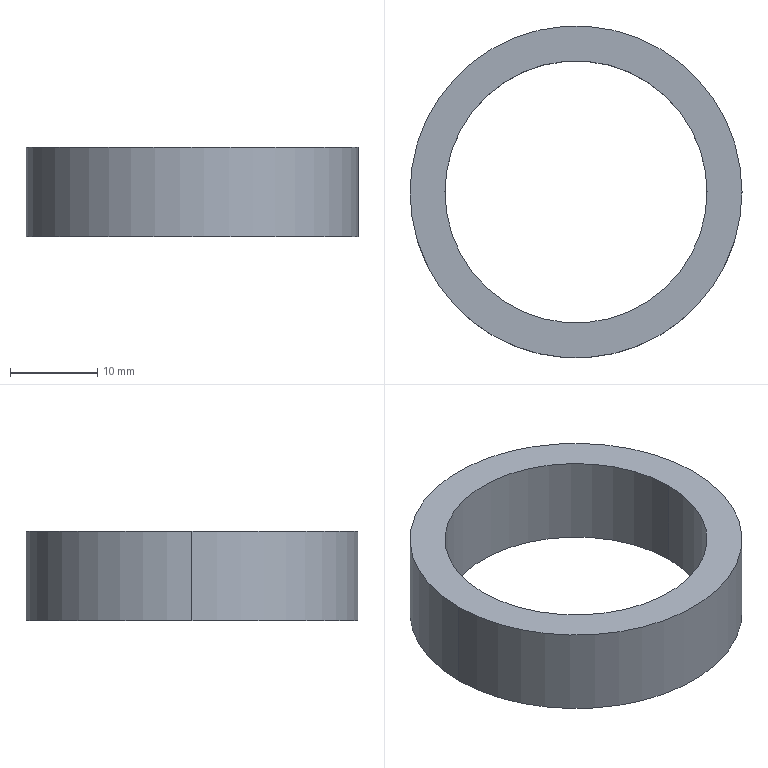Part | SolidWorks | features BaseBody 1 | 1 solid | 6 faces | box 38 x 38 x 10.3 mm | volume 4401 mm3 | cylinder 4 | plane 2 | commonest cylinder face diameters 30 x2 38 x2
STEP:
#1=CARTESIAN_POINT('',(19.,0.,0.));
#2=VERTEX_POINT('',#1);
#3=CARTESIAN_POINT('',(-19.,0.,0.));
#4=VERTEX_POINT('',#3);
#5=CARTESIAN_POINT('',(0.,0.,0.));
#6=DIRECTION('',(0.,0.,1.));
#7=DIRECTION('',(1.,0.,0.));
#8=AXIS2_PLACEMENT_3D('',#5,#6,#7);
#9=CIRCLE('',#8,19.);
#10=EDGE_CURVE('',#2,#4,#9,.T.);
#11=ORIENTED_EDGE('',*,*,#10,.T.);
#12=CARTESIAN_POINT('',(-19.,0.,10.3));
#13=VERTEX_POINT('',#12);
#14=CARTESIAN_POINT('',(-19.,0.,0.));
#15=DIRECTION('',(0.,0.,1.));
#16=VECTOR('',#15,1000.);
#17=LINE('',#14,#16);
#18=EDGE_CURVE('',#4,#13,#17,.T.);
#19=ORIENTED_EDGE('',*,*,#18,.T.);
#20=CARTESIAN_POINT('',(19.,0.,10.3));
#21=VERTEX_POINT('',#20);
#22=CARTESIAN_POINT('',(0.,0.,10.3));
#23=DIRECTION('',(0.,0.,-1.));
#24=DIRECTION('',(1.,0.,0.));
#25=AXIS2_PLACEMENT_3D('',#22,#23,#24);
#26=CIRCLE('',#25,19.);
#27=EDGE_CURVE('',#13,#21,#26,.T.);
#28=ORIENTED_EDGE('',*,*,#27,.T.);
#29=CARTESIAN_POINT('',(19.,0.,0.));
#30=DIRECTION('',(0.,0.,1.));
#31=VECTOR('',#30,1000.);
#32=LINE('',#29,#31);
#33=EDGE_CURVE('',#2,#21,#32,.T.);
#34=ORIENTED_EDGE('',*,*,#33,.F.);
#35=EDGE_LOOP('',(#11,#19,#28,#34));
#36=FACE_OUTER_BOUND('',#35,.T.);
#37=CARTESIAN_POINT('',(0.,0.,0.));
#38=DIRECTION('',(0.,0.,1.));
#39=DIRECTION('',(1.,0.,0.));
#40=AXIS2_PLACEMENT_3D('',#37,#38,#39);
#41=CYLINDRICAL_SURFACE('',#40,19.);
#42=ADVANCED_FACE('',(#36),#41,.T.);
#43=CARTESIAN_POINT('',(15.,0.,0.));
#44=VERTEX_POINT('',#43);
#45=CARTESIAN_POINT('',(-15.,0.,0.));
#46=VERTEX_POINT('',#45);
#47=CARTESIAN_POINT('',(0.,0.,0.));
#48=DIRECTION('',(0.,0.,-1.));
#49=DIRECTION('',(1.,0.,0.));
#50=AXIS2_PLACEMENT_3D('',#47,#48,#49);
#51=CIRCLE('',#50,15.);
#52=EDGE_CURVE('',#44,#46,#51,.T.);
#53=ORIENTED_EDGE('',*,*,#52,.T.);
#54=CARTESIAN_POINT('',(-15.,0.,10.3));
#55=VERTEX_POINT('',#54);
#56=CARTESIAN_POINT('',(-15.,0.,0.));
#57=DIRECTION('',(0.,0.,1.));
#58=VECTOR('',#57,1000.);
#59=LINE('',#56,#58);
#60=EDGE_CURVE('',#46,#55,#59,.T.);
#61=ORIENTED_EDGE('',*,*,#60,.T.);
#62=CARTESIAN_POINT('',(15.,0.,10.3));
#63=VERTEX_POINT('',#62);
#64=CARTESIAN_POINT('',(0.,0.,10.3));
#65=DIRECTION('',(0.,0.,-1.));
#66=DIRECTION('',(1.,0.,0.));
#67=AXIS2_PLACEMENT_3D('',#64,#65,#66);
#68=CIRCLE('',#67,15.);
#69=EDGE_CURVE('',#63,#55,#68,.T.);
#70=ORIENTED_EDGE('',*,*,#69,.F.);
#71=CARTESIAN_POINT('',(15.,0.,0.));
#72=DIRECTION('',(0.,0.,1.));
#73=VECTOR('',#72,1000.);
#74=LINE('',#71,#73);
#75=EDGE_CURVE('',#44,#63,#74,.T.);
#76=ORIENTED_EDGE('',*,*,#75,.F.);
#77=EDGE_LOOP('',(#53,#61,#70,#76));
#78=FACE_OUTER_BOUND('',#77,.T.);
#79=CARTESIAN_POINT('',(0.,0.,0.));
#80=DIRECTION('',(0.,0.,1.));
#81=DIRECTION('',(1.,0.,0.));
#82=AXIS2_PLACEMENT_3D('',#79,#80,#81);
#83=CYLINDRICAL_SURFACE('',#82,15.);
#84=ADVANCED_FACE('',(#78),#83,.F.);
#85=ORIENTED_EDGE('',*,*,#18,.F.);
#86=CARTESIAN_POINT('',(0.,0.,0.));
#87=DIRECTION('',(0.,0.,1.));
#88=DIRECTION('',(1.,0.,0.));
#89=AXIS2_PLACEMENT_3D('',#86,#87,#88);
#90=CIRCLE('',#89,19.);
#91=EDGE_CURVE('',#4,#2,#90,.T.);
#92=ORIENTED_EDGE('',*,*,#91,.T.);
#93=ORIENTED_EDGE('',*,*,#33,.T.);
#94=CARTESIAN_POINT('',(0.,0.,10.3));
#95=DIRECTION('',(0.,0.,-1.));
#96=DIRECTION('',(1.,0.,0.));
#97=AXIS2_PLACEMENT_3D('',#94,#95,#96);
#98=CIRCLE('',#97,19.);
#99=EDGE_CURVE('',#21,#13,#98,.T.);
#100=ORIENTED_EDGE('',*,*,#99,.T.);
#101=EDGE_LOOP('',(#85,#92,#93,#100));
#102=FACE_OUTER_BOUND('',#101,.T.);
#103=CARTESIAN_POINT('',(0.,0.,0.));
#104=DIRECTION('',(0.,0.,1.));
#105=DIRECTION('',(1.,0.,0.));
#106=AXIS2_PLACEMENT_3D('',#103,#104,#105);
#107=CYLINDRICAL_SURFACE('',#106,19.);
#108=ADVANCED_FACE('',(#102),#107,.T.);
#109=ORIENTED_EDGE('',*,*,#52,.F.);
#110=CARTESIAN_POINT('',(0.,0.,0.));
#111=DIRECTION('',(0.,0.,-1.));
#112=DIRECTION('',(1.,0.,0.));
#113=AXIS2_PLACEMENT_3D('',#110,#111,#112);
#114=CIRCLE('',#113,15.);
#115=EDGE_CURVE('',#46,#44,#114,.T.);
#116=ORIENTED_EDGE('',*,*,#115,.F.);
#117=EDGE_LOOP('',(#109,#116));
#118=FACE_BOUND('',#117,.T.);
#119=ORIENTED_EDGE('',*,*,#10,.F.);
#120=ORIENTED_EDGE('',*,*,#91,.F.);
#121=EDGE_LOOP('',(#119,#120));
#122=FACE_OUTER_BOUND('',#121,.T.);
#123=CARTESIAN_POINT('',(0.,0.,0.));
#124=DIRECTION('',(0.,0.,1.));
#125=DIRECTION('',(1.,0.,0.));
#126=AXIS2_PLACEMENT_3D('',#123,#124,#125);
#127=PLANE('',#126);
#128=ADVANCED_FACE('',(#118,#122),#127,.F.);
#129=ORIENTED_EDGE('',*,*,#69,.T.);
#130=CARTESIAN_POINT('',(0.,0.,10.3));
#131=DIRECTION('',(0.,0.,-1.));
#132=DIRECTION('',(1.,0.,0.));
#133=AXIS2_PLACEMENT_3D('',#130,#131,#132);
#134=CIRCLE('',#133,15.);
#135=EDGE_CURVE('',#55,#63,#134,.T.);
#136=ORIENTED_EDGE('',*,*,#135,.T.);
#137=EDGE_LOOP('',(#129,#136));
#138=FACE_BOUND('',#137,.T.);
#139=ORIENTED_EDGE('',*,*,#99,.F.);
#140=ORIENTED_EDGE('',*,*,#27,.F.);
#141=EDGE_LOOP('',(#139,#140));
#142=FACE_OUTER_BOUND('',#141,.T.);
#143=CARTESIAN_POINT('',(0.,0.,10.3));
#144=DIRECTION('',(0.,0.,1.));
#145=DIRECTION('',(1.,0.,0.));
#146=AXIS2_PLACEMENT_3D('',#143,#144,#145);
#147=PLANE('',#146);
#148=ADVANCED_FACE('',(#138,#142),#147,.T.);
#149=ORIENTED_EDGE('',*,*,#60,.F.);
#150=ORIENTED_EDGE('',*,*,#115,.T.);
#151=ORIENTED_EDGE('',*,*,#75,.T.);
#152=ORIENTED_EDGE('',*,*,#135,.F.);
#153=EDGE_LOOP('',(#149,#150,#151,#152));
#154=FACE_OUTER_BOUND('',#153,.T.);
#155=CARTESIAN_POINT('',(0.,0.,0.));
#156=DIRECTION('',(0.,0.,1.));
#157=DIRECTION('',(1.,0.,0.));
#158=AXIS2_PLACEMENT_3D('',#155,#156,#157);
#159=CYLINDRICAL_SURFACE('',#158,15.);
#160=ADVANCED_FACE('',(#154),#159,.F.);
#161=CLOSED_SHELL('',(#42,#84,#108,#128,#148,#160));
#162=MANIFOLD_SOLID_BREP('',#161);
#163=CARTESIAN_POINT('',(0.,0.,0.));
#164=DIRECTION('',(0.,0.,1.));
#165=DIRECTION('',(1.,0.,0.));
#166=AXIS2_PLACEMENT_3D('',#163,#164,#165);
#167=(LENGTH_UNIT()NAMED_UNIT(*)SI_UNIT(.MILLI.,.METRE.));
#168=UNCERTAINTY_MEASURE_WITH_UNIT(LENGTH_MEASURE(0.00001),#167,'','');
#169=(NAMED_UNIT(*)PLANE_ANGLE_UNIT()SI_UNIT($,.RADIAN.));
#170=(NAMED_UNIT(*)SI_UNIT($,.STERADIAN.)SOLID_ANGLE_UNIT());
#171=(GEOMETRIC_REPRESENTATION_CONTEXT(3)GLOBAL_UNCERTAINTY_ASSIGNED_CONTEXT((#168))GLOBAL_UNIT_ASSIGNED_CONTEXT((#167,#169,#170))REPRESENTATION_CONTEXT('',''));
#172=ADVANCED_BREP_SHAPE_REPRESENTATION('',(#162,#166),#171);